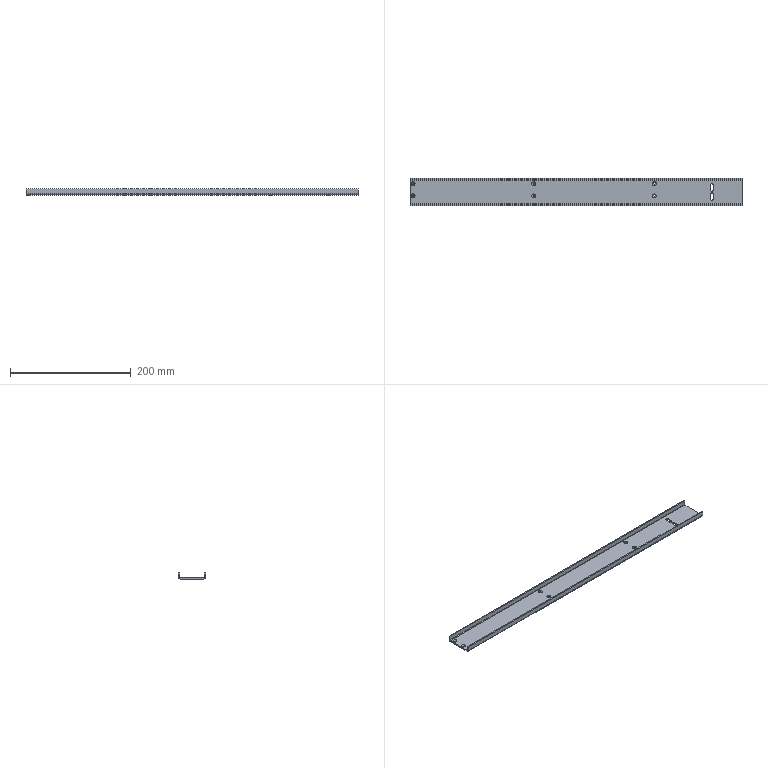Part | SolidWorks | features EdgeFlange 1, FlatPattern 1, HoleWzd 1, ICE 1, SMBaseFlange 1, SheetMetal 1 | 1 solid | 54 faces | box 550 x 45 x 10 mm | volume 65036 mm3 | plane 22 | cylinder 20 | cone 12 | commonest cylinder face diameters 3.4 x12 4.5 x4 1.473 x2 5.473 x2
STEP:
#1=CARTESIAN_POINT('',(-271.7,13.5,-1.6));
#2=VERTEX_POINT('',#1);
#3=CARTESIAN_POINT('',(-268.3,13.5,-1.6));
#4=VERTEX_POINT('',#3);
#5=CARTESIAN_POINT('',(-270.,13.5,-1.6));
#6=DIRECTION('',(0.,0.,1.));
#7=DIRECTION('',(1.,0.,0.));
#8=AXIS2_PLACEMENT_3D('',#5,#6,#7);
#9=CIRCLE('',#8,1.7);
#10=EDGE_CURVE('',#2,#4,#9,.T.);
#11=ORIENTED_EDGE('',*,*,#10,.F.);
#12=CARTESIAN_POINT('',(-273.3,13.5,0.));
#13=VERTEX_POINT('',#12);
#14=CARTESIAN_POINT('',(-273.3,13.5,0.));
#15=DIRECTION('',(-0.7071,0.,0.7071));
#16=VECTOR('',#15,1000.);
#17=LINE('',#14,#16);
#18=EDGE_CURVE('',#2,#13,#17,.T.);
#19=ORIENTED_EDGE('',*,*,#18,.T.);
#20=CARTESIAN_POINT('',(-266.7,13.5,0.));
#21=VERTEX_POINT('',#20);
#22=CARTESIAN_POINT('',(-270.,13.5,0.));
#23=DIRECTION('',(0.,0.,1.));
#24=DIRECTION('',(1.,0.,0.));
#25=AXIS2_PLACEMENT_3D('',#22,#23,#24);
#26=CIRCLE('',#25,3.3);
#27=EDGE_CURVE('',#13,#21,#26,.T.);
#28=ORIENTED_EDGE('',*,*,#27,.T.);
#29=CARTESIAN_POINT('',(-266.7,13.5,0.));
#30=DIRECTION('',(0.7071,0.,0.7071));
#31=VECTOR('',#30,1000.);
#32=LINE('',#29,#31);
#33=EDGE_CURVE('',#4,#21,#32,.T.);
#34=ORIENTED_EDGE('',*,*,#33,.F.);
#35=EDGE_LOOP('',(#11,#19,#28,#34));
#36=FACE_OUTER_BOUND('',#35,.T.);
#37=CARTESIAN_POINT('',(-270.,13.5,0.));
#38=DIRECTION('',(0.,0.,1.));
#39=DIRECTION('',(1.,0.,0.));
#40=AXIS2_PLACEMENT_3D('',#37,#38,#39);
#41=CONICAL_SURFACE('',#40,3.3,0.7854);
#42=ADVANCED_FACE('',(#36),#41,.F.);
#43=CARTESIAN_POINT('',(-271.7,13.5,-2.));
#44=VERTEX_POINT('',#43);
#45=CARTESIAN_POINT('',(-268.3,13.5,-2.));
#46=VERTEX_POINT('',#45);
#47=CARTESIAN_POINT('',(-270.,13.5,-2.));
#48=DIRECTION('',(0.,0.,1.));
#49=DIRECTION('',(1.,0.,0.));
#50=AXIS2_PLACEMENT_3D('',#47,#48,#49);
#51=CIRCLE('',#50,1.7);
#52=EDGE_CURVE('',#44,#46,#51,.T.);
#53=ORIENTED_EDGE('',*,*,#52,.F.);
#54=CARTESIAN_POINT('',(-271.7,13.5,0.));
#55=DIRECTION('',(0.,0.,1.));
#56=VECTOR('',#55,1000.);
#57=LINE('',#54,#56);
#58=EDGE_CURVE('',#44,#2,#57,.T.);
#59=ORIENTED_EDGE('',*,*,#58,.T.);
#60=ORIENTED_EDGE('',*,*,#10,.T.);
#61=CARTESIAN_POINT('',(-268.3,13.5,0.));
#62=DIRECTION('',(0.,0.,1.));
#63=VECTOR('',#62,1000.);
#64=LINE('',#61,#63);
#65=EDGE_CURVE('',#46,#4,#64,.T.);
#66=ORIENTED_EDGE('',*,*,#65,.F.);
#67=EDGE_LOOP('',(#53,#59,#60,#66));
#68=FACE_OUTER_BOUND('',#67,.T.);
#69=CARTESIAN_POINT('',(-270.,13.5,0.));
#70=DIRECTION('',(0.,0.,1.));
#71=DIRECTION('',(1.,0.,0.));
#72=AXIS2_PLACEMENT_3D('',#69,#70,#71);
#73=CYLINDRICAL_SURFACE('',#72,1.7);
#74=ADVANCED_FACE('',(#68),#73,.F.);
#75=CARTESIAN_POINT('',(-271.7,-6.5,-1.6));
#76=VERTEX_POINT('',#75);
#77=CARTESIAN_POINT('',(-268.3,-6.5,-1.6));
#78=VERTEX_POINT('',#77);
#79=CARTESIAN_POINT('',(-270.,-6.5,-1.6));
#80=DIRECTION('',(0.,0.,1.));
#81=DIRECTION('',(1.,0.,0.));
#82=AXIS2_PLACEMENT_3D('',#79,#80,#81);
#83=CIRCLE('',#82,1.7);
#84=EDGE_CURVE('',#76,#78,#83,.T.);
#85=ORIENTED_EDGE('',*,*,#84,.F.);
#86=CARTESIAN_POINT('',(-273.3,-6.5,0.));
#87=VERTEX_POINT('',#86);
#88=CARTESIAN_POINT('',(-273.3,-6.5,0.));
#89=DIRECTION('',(-0.7071,0.,0.7071));
#90=VECTOR('',#89,1000.);
#91=LINE('',#88,#90);
#92=EDGE_CURVE('',#76,#87,#91,.T.);
#93=ORIENTED_EDGE('',*,*,#92,.T.);
#94=CARTESIAN_POINT('',(-266.7,-6.5,0.));
#95=VERTEX_POINT('',#94);
#96=CARTESIAN_POINT('',(-270.,-6.5,0.));
#97=DIRECTION('',(0.,0.,1.));
#98=DIRECTION('',(1.,0.,0.));
#99=AXIS2_PLACEMENT_3D('',#96,#97,#98);
#100=CIRCLE('',#99,3.3);
#101=EDGE_CURVE('',#87,#95,#100,.T.);
#102=ORIENTED_EDGE('',*,*,#101,.T.);
#103=CARTESIAN_POINT('',(-266.7,-6.5,0.));
#104=DIRECTION('',(0.7071,0.,0.7071));
#105=VECTOR('',#104,1000.);
#106=LINE('',#103,#105);
#107=EDGE_CURVE('',#78,#95,#106,.T.);
#108=ORIENTED_EDGE('',*,*,#107,.F.);
#109=EDGE_LOOP('',(#85,#93,#102,#108));
#110=FACE_OUTER_BOUND('',#109,.T.);
#111=CARTESIAN_POINT('',(-270.,-6.5,0.));
#112=DIRECTION('',(0.,0.,1.));
#113=DIRECTION('',(1.,0.,0.));
#114=AXIS2_PLACEMENT_3D('',#111,#112,#113);
#115=CONICAL_SURFACE('',#114,3.3,0.7854);
#116=ADVANCED_FACE('',(#110),#115,.F.);
#117=CARTESIAN_POINT('',(-271.7,-6.5,-2.));
#118=VERTEX_POINT('',#117);
#119=CARTESIAN_POINT('',(-268.3,-6.5,-2.));
#120=VERTEX_POINT('',#119);
#121=CARTESIAN_POINT('',(-270.,-6.5,-2.));
#122=DIRECTION('',(0.,0.,1.));
#123=DIRECTION('',(1.,0.,0.));
#124=AXIS2_PLACEMENT_3D('',#121,#122,#123);
#125=CIRCLE('',#124,1.7);
#126=EDGE_CURVE('',#118,#120,#125,.T.);
#127=ORIENTED_EDGE('',*,*,#126,.F.);
#128=CARTESIAN_POINT('',(-271.7,-6.5,0.));
#129=DIRECTION('',(0.,0.,1.));
#130=VECTOR('',#129,1000.);
#131=LINE('',#128,#130);
#132=EDGE_CURVE('',#118,#76,#131,.T.);
#133=ORIENTED_EDGE('',*,*,#132,.T.);
#134=ORIENTED_EDGE('',*,*,#84,.T.);
#135=CARTESIAN_POINT('',(-268.3,-6.5,0.));
#136=DIRECTION('',(0.,0.,1.));
#137=VECTOR('',#136,1000.);
#138=LINE('',#135,#137);
#139=EDGE_CURVE('',#120,#78,#138,.T.);
#140=ORIENTED_EDGE('',*,*,#139,.F.);
#141=EDGE_LOOP('',(#127,#133,#134,#140));
#142=FACE_OUTER_BOUND('',#141,.T.);
#143=CARTESIAN_POINT('',(-270.,-6.5,0.));
#144=DIRECTION('',(0.,0.,1.));
#145=DIRECTION('',(1.,0.,0.));
#146=AXIS2_PLACEMENT_3D('',#143,#144,#145);
#147=CYLINDRICAL_SURFACE('',#146,1.7);
#148=ADVANCED_FACE('',(#142),#147,.F.);
#149=CARTESIAN_POINT('',(-71.7,-6.5,-1.6));
#150=VERTEX_POINT('',#149);
#151=CARTESIAN_POINT('',(-68.3,-6.5,-1.6));
#152=VERTEX_POINT('',#151);
#153=CARTESIAN_POINT('',(-70.,-6.5,-1.6));
#154=DIRECTION('',(0.,0.,1.));
#155=DIRECTION('',(1.,0.,0.));
#156=AXIS2_PLACEMENT_3D('',#153,#154,#155);
#157=CIRCLE('',#156,1.7);
#158=EDGE_CURVE('',#150,#152,#157,.T.);
#159=ORIENTED_EDGE('',*,*,#158,.F.);
#160=CARTESIAN_POINT('',(-73.3,-6.5,0.));
#161=VERTEX_POINT('',#160);
#162=CARTESIAN_POINT('',(-73.3,-6.5,0.));
#163=DIRECTION('',(-0.7071,0.,0.7071));
#164=VECTOR('',#163,1000.);
#165=LINE('',#162,#164);
#166=EDGE_CURVE('',#150,#161,#165,.T.);
#167=ORIENTED_EDGE('',*,*,#166,.T.);
#168=CARTESIAN_POINT('',(-66.7,-6.5,0.));
#169=VERTEX_POINT('',#168);
#170=CARTESIAN_POINT('',(-70.,-6.5,0.));
#171=DIRECTION('',(0.,0.,1.));
#172=DIRECTION('',(1.,0.,0.));
#173=AXIS2_PLACEMENT_3D('',#170,#171,#172);
#174=CIRCLE('',#173,3.3);
#175=EDGE_CURVE('',#161,#169,#174,.T.);
#176=ORIENTED_EDGE('',*,*,#175,.T.);
#177=CARTESIAN_POINT('',(-66.7,-6.5,0.));
#178=DIRECTION('',(0.7071,0.,0.7071));
#179=VECTOR('',#178,1000.);
#180=LINE('',#177,#179);
#181=EDGE_CURVE('',#152,#169,#180,.T.);
#182=ORIENTED_EDGE('',*,*,#181,.F.);
#183=EDGE_LOOP('',(#159,#167,#176,#182));
#184=FACE_OUTER_BOUND('',#183,.T.);
#185=CARTESIAN_POINT('',(-70.,-6.5,0.));
#186=DIRECTION('',(0.,0.,1.));
#187=DIRECTION('',(1.,0.,0.));
#188=AXIS2_PLACEMENT_3D('',#185,#186,#187);
#189=CONICAL_SURFACE('',#188,3.3,0.7854);
#190=ADVANCED_FACE('',(#184),#189,.F.);
#191=CARTESIAN_POINT('',(-71.7,-6.5,-2.));
#192=VERTEX_POINT('',#191);
#193=CARTESIAN_POINT('',(-68.3,-6.5,-2.));
#194=VERTEX_POINT('',#193);
#195=CARTESIAN_POINT('',(-70.,-6.5,-2.));
#196=DIRECTION('',(0.,0.,1.));
#197=DIRECTION('',(1.,0.,0.));
#198=AXIS2_PLACEMENT_3D('',#195,#196,#197);
#199=CIRCLE('',#198,1.7);
#200=EDGE_CURVE('',#192,#194,#199,.T.);
#201=ORIENTED_EDGE('',*,*,#200,.F.);
#202=CARTESIAN_POINT('',(-71.7,-6.5,0.));
#203=DIRECTION('',(0.,0.,1.));
#204=VECTOR('',#203,1000.);
#205=LINE('',#202,#204);
#206=EDGE_CURVE('',#192,#150,#205,.T.);
#207=ORIENTED_EDGE('',*,*,#206,.T.);
#208=ORIENTED_EDGE('',*,*,#158,.T.);
#209=CARTESIAN_POINT('',(-68.3,-6.5,0.));
#210=DIRECTION('',(0.,0.,1.));
#211=VECTOR('',#210,1000.);
#212=LINE('',#209,#211);
#213=EDGE_CURVE('',#194,#152,#212,.T.);
#214=ORIENTED_EDGE('',*,*,#213,.F.);
#215=EDGE_LOOP('',(#201,#207,#208,#214));
#216=FACE_OUTER_BOUND('',#215,.T.);
#217=CARTESIAN_POINT('',(-70.,-6.5,0.));
#218=DIRECTION('',(0.,0.,1.));
#219=DIRECTION('',(1.,0.,0.));
#220=AXIS2_PLACEMENT_3D('',#217,#218,#219);
#221=CYLINDRICAL_SURFACE('',#220,1.7);
#222=ADVANCED_FACE('',(#216),#221,.F.);
#223=CARTESIAN_POINT('',(-71.7,13.5,-1.6));
#224=VERTEX_POINT('',#223);
#225=CARTESIAN_POINT('',(-68.3,13.5,-1.6));
#226=VERTEX_POINT('',#225);
#227=CARTESIAN_POINT('',(-70.,13.5,-1.6));
#228=DIRECTION('',(0.,0.,1.));
#229=DIRECTION('',(1.,0.,0.));
#230=AXIS2_PLACEMENT_3D('',#227,#228,#229);
#231=CIRCLE('',#230,1.7);
#232=EDGE_CURVE('',#224,#226,#231,.T.);
#233=ORIENTED_EDGE('',*,*,#232,.F.);
#234=CARTESIAN_POINT('',(-73.3,13.5,0.));
#235=VERTEX_POINT('',#234);
#236=CARTESIAN_POINT('',(-73.3,13.5,0.));
#237=DIRECTION('',(-0.7071,0.,0.7071));
#238=VECTOR('',#237,1000.);
#239=LINE('',#236,#238);
#240=EDGE_CURVE('',#224,#235,#239,.T.);
#241=ORIENTED_EDGE('',*,*,#240,.T.);
#242=CARTESIAN_POINT('',(-66.7,13.5,0.));
#243=VERTEX_POINT('',#242);
#244=CARTESIAN_POINT('',(-70.,13.5,0.));
#245=DIRECTION('',(0.,0.,1.));
#246=DIRECTION('',(1.,0.,0.));
#247=AXIS2_PLACEMENT_3D('',#244,#245,#246);
#248=CIRCLE('',#247,3.3);
#249=EDGE_CURVE('',#235,#243,#248,.T.);
#250=ORIENTED_EDGE('',*,*,#249,.T.);
#251=CARTESIAN_POINT('',(-66.7,13.5,0.));
#252=DIRECTION('',(0.7071,0.,0.7071));
#253=VECTOR('',#252,1000.);
#254=LINE('',#251,#253);
#255=EDGE_CURVE('',#226,#243,#254,.T.);
#256=ORIENTED_EDGE('',*,*,#255,.F.);
#257=EDGE_LOOP('',(#233,#241,#250,#256));
#258=FACE_OUTER_BOUND('',#257,.T.);
#259=CARTESIAN_POINT('',(-70.,13.5,0.));
#260=DIRECTION('',(0.,0.,1.));
#261=DIRECTION('',(1.,0.,0.));
#262=AXIS2_PLACEMENT_3D('',#259,#260,#261);
#263=CONICAL_SURFACE('',#262,3.3,0.7854);
#264=ADVANCED_FACE('',(#258),#263,.F.);
#265=CARTESIAN_POINT('',(-71.7,13.5,-2.));
#266=VERTEX_POINT('',#265);
#267=CARTESIAN_POINT('',(-68.3,13.5,-2.));
#268=VERTEX_POINT('',#267);
#269=CARTESIAN_POINT('',(-70.,13.5,-2.));
#270=DIRECTION('',(0.,0.,1.));
#271=DIRECTION('',(1.,0.,0.));
#272=AXIS2_PLACEMENT_3D('',#269,#270,#271);
#273=CIRCLE('',#272,1.7);
#274=EDGE_CURVE('',#266,#268,#273,.T.);
#275=ORIENTED_EDGE('',*,*,#274,.F.);
#276=CARTESIAN_POINT('',(-71.7,13.5,0.));
#277=DIRECTION('',(0.,0.,1.));
#278=VECTOR('',#277,1000.);
#279=LINE('',#276,#278);
#280=EDGE_CURVE('',#266,#224,#279,.T.);
#281=ORIENTED_EDGE('',*,*,#280,.T.);
#282=ORIENTED_EDGE('',*,*,#232,.T.);
#283=CARTESIAN_POINT('',(-68.3,13.5,0.));
#284=DIRECTION('',(0.,0.,1.));
#285=VECTOR('',#284,1000.);
#286=LINE('',#283,#285);
#287=EDGE_CURVE('',#268,#226,#286,.T.);
#288=ORIENTED_EDGE('',*,*,#287,.F.);
#289=EDGE_LOOP('',(#275,#281,#282,#288));
#290=FACE_OUTER_BOUND('',#289,.T.);
#291=CARTESIAN_POINT('',(-70.,13.5,0.));
#292=DIRECTION('',(0.,0.,1.));
#293=DIRECTION('',(1.,0.,0.));
#294=AXIS2_PLACEMENT_3D('',#291,#292,#293);
#295=CYLINDRICAL_SURFACE('',#294,1.7);
#296=ADVANCED_FACE('',(#290),#295,.F.);
#297=CARTESIAN_POINT('',(128.3,13.5,-1.6));
#298=VERTEX_POINT('',#297);
#299=CARTESIAN_POINT('',(131.7,13.5,-1.6));
#300=VERTEX_POINT('',#299);
#301=CARTESIAN_POINT('',(130.,13.5,-1.6));
#302=DIRECTION('',(0.,0.,1.));
#303=DIRECTION('',(1.,0.,0.));
#304=AXIS2_PLACEMENT_3D('',#301,#302,#303);
#305=CIRCLE('',#304,1.7);
#306=EDGE_CURVE('',#298,#300,#305,.T.);
#307=ORIENTED_EDGE('',*,*,#306,.F.);
#308=CARTESIAN_POINT('',(126.7,13.5,0.));
#309=VERTEX_POINT('',#308);
#310=CARTESIAN_POINT('',(126.7,13.5,0.));
#311=DIRECTION('',(-0.7071,0.,0.7071));
#312=VECTOR('',#311,1000.);
#313=LINE('',#310,#312);
#314=EDGE_CURVE('',#298,#309,#313,.T.);
#315=ORIENTED_EDGE('',*,*,#314,.T.);
#316=CARTESIAN_POINT('',(133.3,13.5,0.));
#317=VERTEX_POINT('',#316);
#318=CARTESIAN_POINT('',(130.,13.5,0.));
#319=DIRECTION('',(0.,0.,1.));
#320=DIRECTION('',(1.,0.,0.));
#321=AXIS2_PLACEMENT_3D('',#318,#319,#320);
#322=CIRCLE('',#321,3.3);
#323=EDGE_CURVE('',#309,#317,#322,.T.);
#324=ORIENTED_EDGE('',*,*,#323,.T.);
#325=CARTESIAN_POINT('',(133.3,13.5,0.));
#326=DIRECTION('',(0.7071,0.,0.7071));
#327=VECTOR('',#326,1000.);
#328=LINE('',#325,#327);
#329=EDGE_CURVE('',#300,#317,#328,.T.);
#330=ORIENTED_EDGE('',*,*,#329,.F.);
#331=EDGE_LOOP('',(#307,#315,#324,#330));
#332=FACE_OUTER_BOUND('',#331,.T.);
#333=CARTESIAN_POINT('',(130.,13.5,0.));
#334=DIRECTION('',(0.,0.,1.));
#335=DIRECTION('',(1.,0.,0.));
#336=AXIS2_PLACEMENT_3D('',#333,#334,#335);
#337=CONICAL_SURFACE('',#336,3.3,0.7854);
#338=ADVANCED_FACE('',(#332),#337,.F.);
#339=CARTESIAN_POINT('',(128.3,13.5,-2.));
#340=VERTEX_POINT('',#339);
#341=CARTESIAN_POINT('',(131.7,13.5,-2.));
#342=VERTEX_POINT('',#341);
#343=CARTESIAN_POINT('',(130.,13.5,-2.));
#344=DIRECTION('',(0.,0.,1.));
#345=DIRECTION('',(1.,0.,0.));
#346=AXIS2_PLACEMENT_3D('',#343,#344,#345);
#347=CIRCLE('',#346,1.7);
#348=EDGE_CURVE('',#340,#342,#347,.T.);
#349=ORIENTED_EDGE('',*,*,#348,.F.);
#350=CARTESIAN_POINT('',(128.3,13.5,0.));
#351=DIRECTION('',(0.,0.,1.));
#352=VECTOR('',#351,1000.);
#353=LINE('',#350,#352);
#354=EDGE_CURVE('',#340,#298,#353,.T.);
#355=ORIENTED_EDGE('',*,*,#354,.T.);
#356=ORIENTED_EDGE('',*,*,#306,.T.);
#357=CARTESIAN_POINT('',(131.7,13.5,0.));
#358=DIRECTION('',(0.,0.,1.));
#359=VECTOR('',#358,1000.);
#360=LINE('',#357,#359);
#361=EDGE_CURVE('',#342,#300,#360,.T.);
#362=ORIENTED_EDGE('',*,*,#361,.F.);
#363=EDGE_LOOP('',(#349,#355,#356,#362));
#364=FACE_OUTER_BOUND('',#363,.T.);
#365=CARTESIAN_POINT('',(130.,13.5,0.));
#366=DIRECTION('',(0.,0.,1.));
#367=DIRECTION('',(1.,0.,0.));
#368=AXIS2_PLACEMENT_3D('',#365,#366,#367);
#369=CYLINDRICAL_SURFACE('',#368,1.7);
#370=ADVANCED_FACE('',(#364),#369,.F.);
#371=CARTESIAN_POINT('',(128.3,-6.5,-1.6));
#372=VERTEX_POINT('',#371);
#373=CARTESIAN_POINT('',(131.7,-6.5,-1.6));
#374=VERTEX_POINT('',#373);
#375=CARTESIAN_POINT('',(130.,-6.5,-1.6));
#376=DIRECTION('',(0.,0.,1.));
#377=DIRECTION('',(1.,0.,0.));
#378=AXIS2_PLACEMENT_3D('',#375,#376,#377);
#379=CIRCLE('',#378,1.7);
#380=EDGE_CURVE('',#372,#374,#379,.T.);
#381=ORIENTED_EDGE('',*,*,#380,.F.);
#382=CARTESIAN_POINT('',(126.7,-6.5,0.));
#383=VERTEX_POINT('',#382);
#384=CARTESIAN_POINT('',(126.7,-6.5,0.));
#385=DIRECTION('',(-0.7071,0.,0.7071));
#386=VECTOR('',#385,1000.);
#387=LINE('',#384,#386);
#388=EDGE_CURVE('',#372,#383,#387,.T.);
#389=ORIENTED_EDGE('',*,*,#388,.T.);
#390=CARTESIAN_POINT('',(133.3,-6.5,0.));
#391=VERTEX_POINT('',#390);
#392=CARTESIAN_POINT('',(130.,-6.5,0.));
#393=DIRECTION('',(0.,0.,1.));
#394=DIRECTION('',(1.,0.,0.));
#395=AXIS2_PLACEMENT_3D('',#392,#393,#394);
#396=CIRCLE('',#395,3.3);
#397=EDGE_CURVE('',#383,#391,#396,.T.);
#398=ORIENTED_EDGE('',*,*,#397,.T.);
#399=CARTESIAN_POINT('',(133.3,-6.5,0.));
#400=DIRECTION('',(0.7071,0.,0.7071));
#401=VECTOR('',#400,1000.);
#402=LINE('',#399,#401);
#403=EDGE_CURVE('',#374,#391,#402,.T.);
#404=ORIENTED_EDGE('',*,*,#403,.F.);
#405=EDGE_LOOP('',(#381,#389,#398,#404));
#406=FACE_OUTER_BOUND('',#405,.T.);
#407=CARTESIAN_POINT('',(130.,-6.5,0.));
#408=DIRECTION('',(0.,0.,1.));
#409=DIRECTION('',(1.,0.,0.));
#410=AXIS2_PLACEMENT_3D('',#407,#408,#409);
#411=CONICAL_SURFACE('',#410,3.3,0.7854);
#412=ADVANCED_FACE('',(#406),#411,.F.);
#413=CARTESIAN_POINT('',(128.3,-6.5,-2.));
#414=VERTEX_POINT('',#413);
#415=CARTESIAN_POINT('',(131.7,-6.5,-2.));
#416=VERTEX_POINT('',#415);
#417=CARTESIAN_POINT('',(130.,-6.5,-2.));
#418=DIRECTION('',(0.,0.,1.));
#419=DIRECTION('',(1.,0.,0.));
#420=AXIS2_PLACEMENT_3D('',#417,#418,#419);
#421=CIRCLE('',#420,1.7);
#422=EDGE_CURVE('',#414,#416,#421,.T.);
#423=ORIENTED_EDGE('',*,*,#422,.F.);
#424=CARTESIAN_POINT('',(128.3,-6.5,0.));
#425=DIRECTION('',(0.,0.,1.));
#426=VECTOR('',#425,1000.);
#427=LINE('',#424,#426);
#428=EDGE_CURVE('',#414,#372,#427,.T.);
#429=ORIENTED_EDGE('',*,*,#428,.T.);
#430=ORIENTED_EDGE('',*,*,#380,.T.);
#431=CARTESIAN_POINT('',(131.7,-6.5,0.));
#432=DIRECTION('',(0.,0.,1.));
#433=VECTOR('',#432,1000.);
#434=LINE('',#431,#433);
#435=EDGE_CURVE('',#416,#374,#434,.T.);
#436=ORIENTED_EDGE('',*,*,#435,.F.);
#437=EDGE_LOOP('',(#423,#429,#430,#436));
#438=FACE_OUTER_BOUND('',#437,.T.);
#439=CARTESIAN_POINT('',(130.,-6.5,0.));
#440=DIRECTION('',(0.,0.,1.));
#441=DIRECTION('',(1.,0.,0.));
#442=AXIS2_PLACEMENT_3D('',#439,#440,#441);
#443=CYLINDRICAL_SURFACE('',#442,1.7);
#444=ADVANCED_FACE('',(#438),#443,.F.);
#445=CARTESIAN_POINT('',(-270.,13.5,-2.));
#446=DIRECTION('',(0.,0.,1.));
#447=DIRECTION('',(1.,0.,0.));
#448=AXIS2_PLACEMENT_3D('',#445,#446,#447);
#449=CIRCLE('',#448,1.7);
#450=EDGE_CURVE('',#46,#44,#449,.T.);
#451=ORIENTED_EDGE('',*,*,#450,.T.);
#452=ORIENTED_EDGE('',*,*,#52,.T.);
#453=EDGE_LOOP('',(#451,#452));
#454=FACE_BOUND('',#453,.T.);
#455=CARTESIAN_POINT('',(-270.,-6.5,-2.));
#456=DIRECTION('',(0.,0.,1.));
#457=DIRECTION('',(1.,0.,0.));
#458=AXIS2_PLACEMENT_3D('',#455,#456,#457);
#459=CIRCLE('',#458,1.7);
#460=EDGE_CURVE('',#120,#118,#459,.T.);
#461=ORIENTED_EDGE('',*,*,#460,.T.);
#462=ORIENTED_EDGE('',*,*,#126,.T.);
#463=EDGE_LOOP('',(#461,#462));
#464=FACE_BOUND('',#463,.T.);
#465=CARTESIAN_POINT('',(-70.,-6.5,-2.));
#466=DIRECTION('',(0.,0.,1.));
#467=DIRECTION('',(1.,0.,0.));
#468=AXIS2_PLACEMENT_3D('',#465,#466,#467);
#469=CIRCLE('',#468,1.7);
#470=EDGE_CURVE('',#194,#192,#469,.T.);
#471=ORIENTED_EDGE('',*,*,#470,.T.);
#472=ORIENTED_EDGE('',*,*,#200,.T.);
#473=EDGE_LOOP('',(#471,#472));
#474=FACE_BOUND('',#473,.T.);
#475=CARTESIAN_POINT('',(-70.,13.5,-2.));
#476=DIRECTION('',(0.,0.,1.));
#477=DIRECTION('',(1.,0.,0.));
#478=AXIS2_PLACEMENT_3D('',#475,#476,#477);
#479=CIRCLE('',#478,1.7);
#480=EDGE_CURVE('',#268,#266,#479,.T.);
#481=ORIENTED_EDGE('',*,*,#480,.T.);
#482=ORIENTED_EDGE('',*,*,#274,.T.);
#483=EDGE_LOOP('',(#481,#482));
#484=FACE_BOUND('',#483,.T.);
#485=CARTESIAN_POINT('',(130.,13.5,-2.));
#486=DIRECTION('',(0.,0.,1.));
#487=DIRECTION('',(1.,0.,0.));
#488=AXIS2_PLACEMENT_3D('',#485,#486,#487);
#489=CIRCLE('',#488,1.7);
#490=EDGE_CURVE('',#342,#340,#489,.T.);
#491=ORIENTED_EDGE('',*,*,#490,.T.);
#492=ORIENTED_EDGE('',*,*,#348,.T.);
#493=EDGE_LOOP('',(#491,#492));
#494=FACE_BOUND('',#493,.T.);
#495=CARTESIAN_POINT('',(130.,-6.5,-2.));
#496=DIRECTION('',(0.,0.,1.));
#497=DIRECTION('',(1.,0.,0.));
#498=AXIS2_PLACEMENT_3D('',#495,#496,#497);
#499=CIRCLE('',#498,1.7);
#500=EDGE_CURVE('',#416,#414,#499,.T.);
#501=ORIENTED_EDGE('',*,*,#500,.T.);
#502=ORIENTED_EDGE('',*,*,#422,.T.);
#503=EDGE_LOOP('',(#501,#502));
#504=FACE_BOUND('',#503,.T.);
#505=CARTESIAN_POINT('',(227.25,-11.5,-2.));
#506=VERTEX_POINT('',#505);
#507=CARTESIAN_POINT('',(227.25,-3.5,-2.));
#508=VERTEX_POINT('',#507);
#509=CARTESIAN_POINT('',(227.25,0.,-2.));
#510=DIRECTION('',(0.,1.,0.));
#511=VECTOR('',#510,1000.);
#512=LINE('',#509,#511);
#513=EDGE_CURVE('',#506,#508,#512,.T.);
#514=ORIENTED_EDGE('',*,*,#513,.T.);
#515=CARTESIAN_POINT('',(222.75,-3.5,-2.));
#516=VERTEX_POINT('',#515);
#517=CARTESIAN_POINT('',(225.,-3.5,-2.));
#518=DIRECTION('',(0.,0.,1.));
#519=DIRECTION('',(1.,0.,0.));
#520=AXIS2_PLACEMENT_3D('',#517,#518,#519);
#521=CIRCLE('',#520,2.25);
#522=EDGE_CURVE('',#508,#516,#521,.T.);
#523=ORIENTED_EDGE('',*,*,#522,.T.);
#524=CARTESIAN_POINT('',(222.75,-11.5,-2.));
#525=VERTEX_POINT('',#524);
#526=CARTESIAN_POINT('',(222.75,0.,-2.));
#527=DIRECTION('',(0.,-1.,0.));
#528=VECTOR('',#527,1000.);
#529=LINE('',#526,#528);
#530=EDGE_CURVE('',#516,#525,#529,.T.);
#531=ORIENTED_EDGE('',*,*,#530,.T.);
#532=CARTESIAN_POINT('',(225.,-11.5,-2.));
#533=DIRECTION('',(0.,0.,1.));
#534=DIRECTION('',(1.,0.,0.));
#535=AXIS2_PLACEMENT_3D('',#532,#533,#534);
#536=CIRCLE('',#535,2.25);
#537=EDGE_CURVE('',#525,#506,#536,.T.);
#538=ORIENTED_EDGE('',*,*,#537,.T.);
#539=EDGE_LOOP('',(#514,#523,#531,#538));
#540=FACE_BOUND('',#539,.T.);
#541=CARTESIAN_POINT('',(227.25,3.5,-2.));
#542=VERTEX_POINT('',#541);
#543=CARTESIAN_POINT('',(227.25,11.5,-2.));
#544=VERTEX_POINT('',#543);
#545=CARTESIAN_POINT('',(227.25,0.,-2.));
#546=DIRECTION('',(0.,1.,0.));
#547=VECTOR('',#546,1000.);
#548=LINE('',#545,#547);
#549=EDGE_CURVE('',#542,#544,#548,.T.);
#550=ORIENTED_EDGE('',*,*,#549,.T.);
#551=CARTESIAN_POINT('',(222.75,11.5,-2.));
#552=VERTEX_POINT('',#551);
#553=CARTESIAN_POINT('',(225.,11.5,-2.));
#554=DIRECTION('',(0.,0.,1.));
#555=DIRECTION('',(1.,0.,0.));
#556=AXIS2_PLACEMENT_3D('',#553,#554,#555);
#557=CIRCLE('',#556,2.25);
#558=EDGE_CURVE('',#544,#552,#557,.T.);
#559=ORIENTED_EDGE('',*,*,#558,.T.);
#560=CARTESIAN_POINT('',(222.75,3.5,-2.));
#561=VERTEX_POINT('',#560);
#562=CARTESIAN_POINT('',(222.75,0.,-2.));
#563=DIRECTION('',(0.,-1.,0.));
#564=VECTOR('',#563,1000.);
#565=LINE('',#562,#564);
#566=EDGE_CURVE('',#552,#561,#565,.T.);
#567=ORIENTED_EDGE('',*,*,#566,.T.);
#568=CARTESIAN_POINT('',(225.,3.5,-2.));
#569=DIRECTION('',(0.,0.,1.));
#570=DIRECTION('',(1.,0.,0.));
#571=AXIS2_PLACEMENT_3D('',#568,#569,#570);
#572=CIRCLE('',#571,2.25);
#573=EDGE_CURVE('',#561,#542,#572,.T.);
#574=ORIENTED_EDGE('',*,*,#573,.T.);
#575=EDGE_LOOP('',(#550,#559,#567,#574));
#576=FACE_BOUND('',#575,.T.);
#577=CARTESIAN_POINT('',(-275.,19.763,-2.));
#578=VERTEX_POINT('',#577);
#579=CARTESIAN_POINT('',(275.,19.763,-2.));
#580=VERTEX_POINT('',#579);
#581=CARTESIAN_POINT('',(-275.,19.763,-2.));
#582=DIRECTION('',(1.,0.,0.));
#583=VECTOR('',#582,1000.);
#584=LINE('',#581,#583);
#585=EDGE_CURVE('',#578,#580,#584,.T.);
#586=ORIENTED_EDGE('',*,*,#585,.T.);
#587=CARTESIAN_POINT('',(275.,-19.763,-2.));
#588=VERTEX_POINT('',#587);
#589=CARTESIAN_POINT('',(275.,22.5,-2.));
#590=DIRECTION('',(0.,1.,0.));
#591=VECTOR('',#590,1000.);
#592=LINE('',#589,#591);
#593=EDGE_CURVE('',#588,#580,#592,.T.);
#594=ORIENTED_EDGE('',*,*,#593,.F.);
#595=CARTESIAN_POINT('',(-275.,-19.763,-2.));
#596=VERTEX_POINT('',#595);
#597=CARTESIAN_POINT('',(275.,-19.763,-2.));
#598=DIRECTION('',(-1.,0.,0.));
#599=VECTOR('',#598,1000.);
#600=LINE('',#597,#599);
#601=EDGE_CURVE('',#588,#596,#600,.T.);
#602=ORIENTED_EDGE('',*,*,#601,.T.);
#603=CARTESIAN_POINT('',(-275.,22.5,-2.));
#604=DIRECTION('',(0.,-1.,0.));
#605=VECTOR('',#604,1000.);
#606=LINE('',#603,#605);
#607=EDGE_CURVE('',#578,#596,#606,.T.);
#608=ORIENTED_EDGE('',*,*,#607,.F.);
#609=EDGE_LOOP('',(#586,#594,#602,#608));
#610=FACE_OUTER_BOUND('',#609,.T.);
#611=CARTESIAN_POINT('',(0.,0.,-2.));
#612=DIRECTION('',(0.,0.,1.));
#613=DIRECTION('',(1.,0.,0.));
#614=AXIS2_PLACEMENT_3D('',#611,#612,#613);
#615=PLANE('',#614);
#616=ADVANCED_FACE('',(#454,#464,#474,#484,#494,#504,#540,#576,#610),#615,.F.);
#617=CARTESIAN_POINT('',(-270.,13.5,0.));
#618=DIRECTION('',(0.,0.,1.));
#619=DIRECTION('',(1.,0.,0.));
#620=AXIS2_PLACEMENT_3D('',#617,#618,#619);
#621=CIRCLE('',#620,3.3);
#622=EDGE_CURVE('',#21,#13,#621,.T.);
#623=ORIENTED_EDGE('',*,*,#622,.F.);
#624=ORIENTED_EDGE('',*,*,#27,.F.);
#625=EDGE_LOOP('',(#623,#624));
#626=FACE_BOUND('',#625,.T.);
#627=CARTESIAN_POINT('',(-270.,-6.5,0.));
#628=DIRECTION('',(0.,0.,1.));
#629=DIRECTION('',(1.,0.,0.));
#630=AXIS2_PLACEMENT_3D('',#627,#628,#629);
#631=CIRCLE('',#630,3.3);
#632=EDGE_CURVE('',#95,#87,#631,.T.);
#633=ORIENTED_EDGE('',*,*,#632,.F.);
#634=ORIENTED_EDGE('',*,*,#101,.F.);
#635=EDGE_LOOP('',(#633,#634));
#636=FACE_BOUND('',#635,.T.);
#637=CARTESIAN_POINT('',(-70.,-6.5,0.));
#638=DIRECTION('',(0.,0.,1.));
#639=DIRECTION('',(1.,0.,0.));
#640=AXIS2_PLACEMENT_3D('',#637,#638,#639);
#641=CIRCLE('',#640,3.3);
#642=EDGE_CURVE('',#169,#161,#641,.T.);
#643=ORIENTED_EDGE('',*,*,#642,.F.);
#644=ORIENTED_EDGE('',*,*,#175,.F.);
#645=EDGE_LOOP('',(#643,#644));
#646=FACE_BOUND('',#645,.T.);
#647=CARTESIAN_POINT('',(-70.,13.5,0.));
#648=DIRECTION('',(0.,0.,1.));
#649=DIRECTION('',(1.,0.,0.));
#650=AXIS2_PLACEMENT_3D('',#647,#648,#649);
#651=CIRCLE('',#650,3.3);
#652=EDGE_CURVE('',#243,#235,#651,.T.);
#653=ORIENTED_EDGE('',*,*,#652,.F.);
#654=ORIENTED_EDGE('',*,*,#249,.F.);
#655=EDGE_LOOP('',(#653,#654));
#656=FACE_BOUND('',#655,.T.);
#657=CARTESIAN_POINT('',(130.,13.5,0.));
#658=DIRECTION('',(0.,0.,1.));
#659=DIRECTION('',(1.,0.,0.));
#660=AXIS2_PLACEMENT_3D('',#657,#658,#659);
#661=CIRCLE('',#660,3.3);
#662=EDGE_CURVE('',#317,#309,#661,.T.);
#663=ORIENTED_EDGE('',*,*,#662,.F.);
#664=ORIENTED_EDGE('',*,*,#323,.F.);
#665=EDGE_LOOP('',(#663,#664));
#666=FACE_BOUND('',#665,.T.);
#667=CARTESIAN_POINT('',(130.,-6.5,0.));
#668=DIRECTION('',(0.,0.,1.));
#669=DIRECTION('',(1.,0.,0.));
#670=AXIS2_PLACEMENT_3D('',#667,#668,#669);
#671=CIRCLE('',#670,3.3);
#672=EDGE_CURVE('',#391,#383,#671,.T.);
#673=ORIENTED_EDGE('',*,*,#672,.F.);
#674=ORIENTED_EDGE('',*,*,#397,.F.);
#675=EDGE_LOOP('',(#673,#674));
#676=FACE_BOUND('',#675,.T.);
#677=CARTESIAN_POINT('',(227.25,-3.5,0.));
#678=VERTEX_POINT('',#677);
#679=CARTESIAN_POINT('',(222.75,-3.5,0.));
#680=VERTEX_POINT('',#679);
#681=CARTESIAN_POINT('',(225.,-3.5,0.));
#682=DIRECTION('',(0.,0.,1.));
#683=DIRECTION('',(1.,0.,0.));
#684=AXIS2_PLACEMENT_3D('',#681,#682,#683);
#685=CIRCLE('',#684,2.25);
#686=EDGE_CURVE('',#678,#680,#685,.T.);
#687=ORIENTED_EDGE('',*,*,#686,.F.);
#688=CARTESIAN_POINT('',(227.25,-11.5,0.));
#689=VERTEX_POINT('',#688);
#690=CARTESIAN_POINT('',(227.25,-3.5,0.));
#691=DIRECTION('',(0.,1.,0.));
#692=VECTOR('',#691,1000.);
#693=LINE('',#690,#692);
#694=EDGE_CURVE('',#689,#678,#693,.T.);
#695=ORIENTED_EDGE('',*,*,#694,.F.);
#696=CARTESIAN_POINT('',(222.75,-11.5,0.));
#697=VERTEX_POINT('',#696);
#698=CARTESIAN_POINT('',(225.,-11.5,0.));
#699=DIRECTION('',(0.,0.,1.));
#700=DIRECTION('',(1.,0.,0.));
#701=AXIS2_PLACEMENT_3D('',#698,#699,#700);
#702=CIRCLE('',#701,2.25);
#703=EDGE_CURVE('',#697,#689,#702,.T.);
#704=ORIENTED_EDGE('',*,*,#703,.F.);
#705=CARTESIAN_POINT('',(222.75,-3.5,0.));
#706=DIRECTION('',(0.,-1.,0.));
#707=VECTOR('',#706,1000.);
#708=LINE('',#705,#707);
#709=EDGE_CURVE('',#680,#697,#708,.T.);
#710=ORIENTED_EDGE('',*,*,#709,.F.);
#711=EDGE_LOOP('',(#687,#695,#704,#710));
#712=FACE_BOUND('',#711,.T.);
#713=CARTESIAN_POINT('',(227.25,11.5,0.));
#714=VERTEX_POINT('',#713);
#715=CARTESIAN_POINT('',(222.75,11.5,0.));
#716=VERTEX_POINT('',#715);
#717=CARTESIAN_POINT('',(225.,11.5,0.));
#718=DIRECTION('',(0.,0.,1.));
#719=DIRECTION('',(1.,0.,0.));
#720=AXIS2_PLACEMENT_3D('',#717,#718,#719);
#721=CIRCLE('',#720,2.25);
#722=EDGE_CURVE('',#714,#716,#721,.T.);
#723=ORIENTED_EDGE('',*,*,#722,.F.);
#724=CARTESIAN_POINT('',(227.25,3.5,0.));
#725=VERTEX_POINT('',#724);
#726=CARTESIAN_POINT('',(227.25,11.5,0.));
#727=DIRECTION('',(0.,1.,0.));
#728=VECTOR('',#727,1000.);
#729=LINE('',#726,#728);
#730=EDGE_CURVE('',#725,#714,#729,.T.);
#731=ORIENTED_EDGE('',*,*,#730,.F.);
#732=CARTESIAN_POINT('',(222.75,3.5,0.));
#733=VERTEX_POINT('',#732);
#734=CARTESIAN_POINT('',(225.,3.5,0.));
#735=DIRECTION('',(0.,0.,1.));
#736=DIRECTION('',(1.,0.,0.));
#737=AXIS2_PLACEMENT_3D('',#734,#735,#736);
#738=CIRCLE('',#737,2.25);
#739=EDGE_CURVE('',#733,#725,#738,.T.);
#740=ORIENTED_EDGE('',*,*,#739,.F.);
#741=CARTESIAN_POINT('',(222.75,11.5,0.));
#742=DIRECTION('',(0.,-1.,0.));
#743=VECTOR('',#742,1000.);
#744=LINE('',#741,#743);
#745=EDGE_CURVE('',#716,#733,#744,.T.);
#746=ORIENTED_EDGE('',*,*,#745,.F.);
#747=EDGE_LOOP('',(#723,#731,#740,#746));
#748=FACE_BOUND('',#747,.T.);
#749=CARTESIAN_POINT('',(275.,-19.763,0.));
#750=VERTEX_POINT('',#749);
#751=CARTESIAN_POINT('',(275.,19.763,0.));
#752=VERTEX_POINT('',#751);
#753=CARTESIAN_POINT('',(275.,22.5,0.));
#754=DIRECTION('',(0.,1.,0.));
#755=VECTOR('',#754,1000.);
#756=LINE('',#753,#755);
#757=EDGE_CURVE('',#750,#752,#756,.T.);
#758=ORIENTED_EDGE('',*,*,#757,.T.);
#759=CARTESIAN_POINT('',(-275.,19.763,0.));
#760=VERTEX_POINT('',#759);
#761=CARTESIAN_POINT('',(-275.,19.763,0.));
#762=DIRECTION('',(1.,0.,0.));
#763=VECTOR('',#762,1000.);
#764=LINE('',#761,#763);
#765=EDGE_CURVE('',#760,#752,#764,.T.);
#766=ORIENTED_EDGE('',*,*,#765,.F.);
#767=CARTESIAN_POINT('',(-275.,-19.763,0.));
#768=VERTEX_POINT('',#767);
#769=CARTESIAN_POINT('',(-275.,22.5,0.));
#770=DIRECTION('',(0.,-1.,0.));
#771=VECTOR('',#770,1000.);
#772=LINE('',#769,#771);
#773=EDGE_CURVE('',#760,#768,#772,.T.);
#774=ORIENTED_EDGE('',*,*,#773,.T.);
#775=CARTESIAN_POINT('',(275.,-19.763,0.));
#776=DIRECTION('',(-1.,0.,0.));
#777=VECTOR('',#776,1000.);
#778=LINE('',#775,#777);
#779=EDGE_CURVE('',#750,#768,#778,.T.);
#780=ORIENTED_EDGE('',*,*,#779,.F.);
#781=EDGE_LOOP('',(#758,#766,#774,#780));
#782=FACE_OUTER_BOUND('',#781,.T.);
#783=CARTESIAN_POINT('',(0.,0.,0.));
#784=DIRECTION('',(0.,0.,1.));
#785=DIRECTION('',(1.,0.,0.));
#786=AXIS2_PLACEMENT_3D('',#783,#784,#785);
#787=PLANE('',#786);
#788=ADVANCED_FACE('',(#626,#636,#646,#656,#666,#676,#712,#748,#782),#787,.T.);
#789=ORIENTED_EDGE('',*,*,#773,.F.);
#790=CARTESIAN_POINT('',(-275.,19.763,0.));
#791=DIRECTION('',(0.,0.,-1.));
#792=VECTOR('',#791,1000.);
#793=LINE('',#790,#792);
#794=EDGE_CURVE('',#760,#578,#793,.T.);
#795=ORIENTED_EDGE('',*,*,#794,.T.);
#796=ORIENTED_EDGE('',*,*,#607,.T.);
#797=CARTESIAN_POINT('',(-275.,-19.763,0.));
#798=DIRECTION('',(0.,0.,-1.));
#799=VECTOR('',#798,1000.);
#800=LINE('',#797,#799);
#801=EDGE_CURVE('',#768,#596,#800,.T.);
#802=ORIENTED_EDGE('',*,*,#801,.F.);
#803=EDGE_LOOP('',(#789,#795,#796,#802));
#804=FACE_OUTER_BOUND('',#803,.T.);
#805=CARTESIAN_POINT('',(-275.,22.5,-2.));
#806=DIRECTION('',(-1.,0.,0.));
#807=DIRECTION('',(0.,0.,1.));
#808=AXIS2_PLACEMENT_3D('',#805,#806,#807);
#809=PLANE('',#808);
#810=ADVANCED_FACE('',(#804),#809,.T.);
#811=CARTESIAN_POINT('',(275.,19.763,0.));
#812=DIRECTION('',(0.,0.,-1.));
#813=VECTOR('',#812,1000.);
#814=LINE('',#811,#813);
#815=EDGE_CURVE('',#752,#580,#814,.T.);
#816=ORIENTED_EDGE('',*,*,#815,.F.);
#817=ORIENTED_EDGE('',*,*,#757,.F.);
#818=CARTESIAN_POINT('',(275.,-19.763,0.));
#819=DIRECTION('',(0.,0.,-1.));
#820=VECTOR('',#819,1000.);
#821=LINE('',#818,#820);
#822=EDGE_CURVE('',#750,#588,#821,.T.);
#823=ORIENTED_EDGE('',*,*,#822,.T.);
#824=ORIENTED_EDGE('',*,*,#593,.T.);
#825=EDGE_LOOP('',(#816,#817,#823,#824));
#826=FACE_OUTER_BOUND('',#825,.T.);
#827=CARTESIAN_POINT('',(275.,22.5,-2.));
#828=DIRECTION('',(1.,0.,0.));
#829=DIRECTION('',(0.,0.,-1.));
#830=AXIS2_PLACEMENT_3D('',#827,#828,#829);
#831=PLANE('',#830);
#832=ADVANCED_FACE('',(#826),#831,.T.);
#833=CARTESIAN_POINT('',(-275.,-20.5,0.7366));
#834=VERTEX_POINT('',#833);
#835=CARTESIAN_POINT('',(-275.,-22.5,0.7366));
#836=VERTEX_POINT('',#835);
#837=CARTESIAN_POINT('',(-275.,-22.5,0.7366));
#838=DIRECTION('',(0.,-1.,0.));
#839=VECTOR('',#838,1000.);
#840=LINE('',#837,#839);
#841=EDGE_CURVE('',#834,#836,#840,.T.);
#842=ORIENTED_EDGE('',*,*,#841,.F.);
#843=CARTESIAN_POINT('',(-275.,-19.763,0.7366));
#844=DIRECTION('',(-1.,0.,0.));
#845=DIRECTION('',(0.,0.,-1.));
#846=AXIS2_PLACEMENT_3D('',#843,#844,#845);
#847=CIRCLE('',#846,0.7366);
#848=EDGE_CURVE('',#768,#834,#847,.T.);
#849=ORIENTED_EDGE('',*,*,#848,.F.);
#850=ORIENTED_EDGE('',*,*,#801,.T.);
#851=CARTESIAN_POINT('',(-275.,-19.763,0.7366));
#852=DIRECTION('',(-1.,0.,0.));
#853=DIRECTION('',(0.,0.,-1.));
#854=AXIS2_PLACEMENT_3D('',#851,#852,#853);
#855=CIRCLE('',#854,2.737);
#856=EDGE_CURVE('',#596,#836,#855,.T.);
#857=ORIENTED_EDGE('',*,*,#856,.T.);
#858=EDGE_LOOP('',(#842,#849,#850,#857));
#859=FACE_OUTER_BOUND('',#858,.T.);
#860=CARTESIAN_POINT('',(-275.,-19.763,0.7366));
#861=DIRECTION('',(-1.,0.,0.));
#862=DIRECTION('',(0.,0.,1.));
#863=AXIS2_PLACEMENT_3D('',#860,#861,#862);
#864=PLANE('',#863);
#865=ADVANCED_FACE('',(#859),#864,.T.);
#866=CARTESIAN_POINT('',(275.,-20.5,0.7366));
#867=VERTEX_POINT('',#866);
#868=CARTESIAN_POINT('',(275.,-19.763,0.7366));
#869=DIRECTION('',(1.,0.,0.));
#870=DIRECTION('',(0.,0.,-1.));
#871=AXIS2_PLACEMENT_3D('',#868,#869,#870);
#872=CIRCLE('',#871,0.7366);
#873=EDGE_CURVE('',#867,#750,#872,.T.);
#874=ORIENTED_EDGE('',*,*,#873,.F.);
#875=CARTESIAN_POINT('',(275.,-22.5,0.7366));
#876=VERTEX_POINT('',#875);
#877=CARTESIAN_POINT('',(275.,-20.5,0.7366));
#878=DIRECTION('',(0.,-1.,0.));
#879=VECTOR('',#878,1000.);
#880=LINE('',#877,#879);
#881=EDGE_CURVE('',#867,#876,#880,.T.);
#882=ORIENTED_EDGE('',*,*,#881,.T.);
#883=CARTESIAN_POINT('',(275.,-19.763,0.7366));
#884=DIRECTION('',(1.,0.,0.));
#885=DIRECTION('',(0.,0.,-1.));
#886=AXIS2_PLACEMENT_3D('',#883,#884,#885);
#887=CIRCLE('',#886,2.737);
#888=EDGE_CURVE('',#876,#588,#887,.T.);
#889=ORIENTED_EDGE('',*,*,#888,.T.);
#890=ORIENTED_EDGE('',*,*,#822,.F.);
#891=EDGE_LOOP('',(#874,#882,#889,#890));
#892=FACE_OUTER_BOUND('',#891,.T.);
#893=CARTESIAN_POINT('',(275.,-19.763,0.7366));
#894=DIRECTION('',(-1.,0.,0.));
#895=DIRECTION('',(0.,0.,1.));
#896=AXIS2_PLACEMENT_3D('',#893,#894,#895);
#897=PLANE('',#896);
#898=ADVANCED_FACE('',(#892),#897,.F.);
#899=ORIENTED_EDGE('',*,*,#601,.F.);
#900=ORIENTED_EDGE('',*,*,#888,.F.);
#901=CARTESIAN_POINT('',(-275.,-22.5,0.7366));
#902=DIRECTION('',(-1.,0.,0.));
#903=VECTOR('',#902,1000.);
#904=LINE('',#901,#903);
#905=EDGE_CURVE('',#876,#836,#904,.T.);
#906=ORIENTED_EDGE('',*,*,#905,.T.);
#907=ORIENTED_EDGE('',*,*,#856,.F.);
#908=EDGE_LOOP('',(#899,#900,#906,#907));
#909=FACE_OUTER_BOUND('',#908,.T.);
#910=CARTESIAN_POINT('',(275.,-19.763,0.7366));
#911=DIRECTION('',(1.,0.,0.));
#912=DIRECTION('',(0.,-1.,0.));
#913=AXIS2_PLACEMENT_3D('',#910,#911,#912);
#914=CYLINDRICAL_SURFACE('',#913,2.737);
#915=ADVANCED_FACE('',(#909),#914,.T.);
#916=ORIENTED_EDGE('',*,*,#779,.T.);
#917=ORIENTED_EDGE('',*,*,#848,.T.);
#918=CARTESIAN_POINT('',(-275.,-20.5,0.7366));
#919=DIRECTION('',(1.,0.,0.));
#920=VECTOR('',#919,1000.);
#921=LINE('',#918,#920);
#922=EDGE_CURVE('',#834,#867,#921,.T.);
#923=ORIENTED_EDGE('',*,*,#922,.T.);
#924=ORIENTED_EDGE('',*,*,#873,.T.);
#925=EDGE_LOOP('',(#916,#917,#923,#924));
#926=FACE_OUTER_BOUND('',#925,.T.);
#927=CARTESIAN_POINT('',(275.,-19.763,0.7366));
#928=DIRECTION('',(1.,0.,0.));
#929=DIRECTION('',(0.,-1.,0.));
#930=AXIS2_PLACEMENT_3D('',#927,#928,#929);
#931=CYLINDRICAL_SURFACE('',#930,0.7366);
#932=ADVANCED_FACE('',(#926),#931,.F.);
#933=ORIENTED_EDGE('',*,*,#841,.T.);
#934=CARTESIAN_POINT('',(-275.,-22.5,8.));
#935=VERTEX_POINT('',#934);
#936=CARTESIAN_POINT('',(-275.,-22.5,0.));
#937=DIRECTION('',(0.,0.,-1.));
#938=VECTOR('',#937,1000.);
#939=LINE('',#936,#938);
#940=EDGE_CURVE('',#935,#836,#939,.T.);
#941=ORIENTED_EDGE('',*,*,#940,.F.);
#942=CARTESIAN_POINT('',(-275.,-20.5,8.));
#943=VERTEX_POINT('',#942);
#944=CARTESIAN_POINT('',(-275.,-22.5,8.));
#945=DIRECTION('',(0.,1.,0.));
#946=VECTOR('',#945,1000.);
#947=LINE('',#944,#946);
#948=EDGE_CURVE('',#935,#943,#947,.T.);
#949=ORIENTED_EDGE('',*,*,#948,.T.);
#950=CARTESIAN_POINT('',(-275.,-20.5,0.));
#951=DIRECTION('',(0.,0.,-1.));
#952=VECTOR('',#951,1000.);
#953=LINE('',#950,#952);
#954=EDGE_CURVE('',#943,#834,#953,.T.);
#955=ORIENTED_EDGE('',*,*,#954,.T.);
#956=EDGE_LOOP('',(#933,#941,#949,#955));
#957=FACE_OUTER_BOUND('',#956,.T.);
#958=CARTESIAN_POINT('',(-275.,-22.5,0.));
#959=DIRECTION('',(1.,0.,0.));
#960=DIRECTION('',(0.,0.,-1.));
#961=AXIS2_PLACEMENT_3D('',#958,#959,#960);
#962=PLANE('',#961);
#963=ADVANCED_FACE('',(#957),#962,.F.);
#964=ORIENTED_EDGE('',*,*,#881,.F.);
#965=CARTESIAN_POINT('',(275.,-20.5,8.));
#966=VERTEX_POINT('',#965);
#967=CARTESIAN_POINT('',(275.,-20.5,8.));
#968=DIRECTION('',(0.,0.,1.));
#969=VECTOR('',#968,1000.);
#970=LINE('',#967,#969);
#971=EDGE_CURVE('',#867,#966,#970,.T.);
#972=ORIENTED_EDGE('',*,*,#971,.T.);
#973=CARTESIAN_POINT('',(275.,-22.5,8.));
#974=VERTEX_POINT('',#973);
#975=CARTESIAN_POINT('',(275.,-22.5,8.));
#976=DIRECTION('',(0.,1.,0.));
#977=VECTOR('',#976,1000.);
#978=LINE('',#975,#977);
#979=EDGE_CURVE('',#974,#966,#978,.T.);
#980=ORIENTED_EDGE('',*,*,#979,.F.);
#981=CARTESIAN_POINT('',(275.,-22.5,0.));
#982=DIRECTION('',(0.,0.,1.));
#983=VECTOR('',#982,1000.);
#984=LINE('',#981,#983);
#985=EDGE_CURVE('',#876,#974,#984,.T.);
#986=ORIENTED_EDGE('',*,*,#985,.F.);
#987=EDGE_LOOP('',(#964,#972,#980,#986));
#988=FACE_OUTER_BOUND('',#987,.T.);
#989=CARTESIAN_POINT('',(275.,-22.5,8.));
#990=DIRECTION('',(-1.,0.,0.));
#991=DIRECTION('',(0.,0.,1.));
#992=AXIS2_PLACEMENT_3D('',#989,#990,#991);
#993=PLANE('',#992);
#994=ADVANCED_FACE('',(#988),#993,.F.);
#995=ORIENTED_EDGE('',*,*,#905,.F.);
#996=ORIENTED_EDGE('',*,*,#985,.T.);
#997=CARTESIAN_POINT('',(0.,-22.5,8.));
#998=DIRECTION('',(-1.,0.,0.));
#999=VECTOR('',#998,1000.);
#1000=LINE('',#997,#999);
#1001=EDGE_CURVE('',#974,#935,#1000,.T.);
#1002=ORIENTED_EDGE('',*,*,#1001,.T.);
#1003=ORIENTED_EDGE('',*,*,#940,.T.);
#1004=EDGE_LOOP('',(#995,#996,#1002,#1003));
#1005=FACE_OUTER_BOUND('',#1004,.T.);
#1006=CARTESIAN_POINT('',(0.,-22.5,0.));
#1007=DIRECTION('',(0.,1.,0.));
#1008=DIRECTION('',(0.,0.,1.));
#1009=AXIS2_PLACEMENT_3D('',#1006,#1007,#1008);
#1010=PLANE('',#1009);
#1011=ADVANCED_FACE('',(#1005),#1010,.F.);
#1012=ORIENTED_EDGE('',*,*,#971,.F.);
#1013=ORIENTED_EDGE('',*,*,#922,.F.);
#1014=ORIENTED_EDGE('',*,*,#954,.F.);
#1015=CARTESIAN_POINT('',(-275.,-20.5,8.));
#1016=DIRECTION('',(-1.,0.,0.));
#1017=VECTOR('',#1016,1000.);
#1018=LINE('',#1015,#1017);
#1019=EDGE_CURVE('',#966,#943,#1018,.T.);
#1020=ORIENTED_EDGE('',*,*,#1019,.F.);
#1021=EDGE_LOOP('',(#1012,#1013,#1014,#1020));
#1022=FACE_OUTER_BOUND('',#1021,.T.);
#1023=CARTESIAN_POINT('',(0.,-20.5,0.));
#1024=DIRECTION('',(0.,1.,0.));
#1025=DIRECTION('',(0.,0.,1.));
#1026=AXIS2_PLACEMENT_3D('',#1023,#1024,#1025);
#1027=PLANE('',#1026);
#1028=ADVANCED_FACE('',(#1022),#1027,.T.);
#1029=ORIENTED_EDGE('',*,*,#1019,.T.);
#1030=ORIENTED_EDGE('',*,*,#948,.F.);
#1031=ORIENTED_EDGE('',*,*,#1001,.F.);
#1032=ORIENTED_EDGE('',*,*,#979,.T.);
#1033=EDGE_LOOP('',(#1029,#1030,#1031,#1032));
#1034=FACE_OUTER_BOUND('',#1033,.T.);
#1035=CARTESIAN_POINT('',(-275.,-22.5,8.));
#1036=DIRECTION('',(0.,0.,-1.));
#1037=DIRECTION('',(0.,1.,0.));
#1038=AXIS2_PLACEMENT_3D('',#1035,#1036,#1037);
#1039=PLANE('',#1038);
#1040=ADVANCED_FACE('',(#1034),#1039,.F.);
#1041=CARTESIAN_POINT('',(275.,20.5,0.7366));
#1042=VERTEX_POINT('',#1041);
#1043=CARTESIAN_POINT('',(275.,22.5,0.7366));
#1044=VERTEX_POINT('',#1043);
#1045=CARTESIAN_POINT('',(275.,22.5,0.7366));
#1046=DIRECTION('',(0.,1.,0.));
#1047=VECTOR('',#1046,1000.);
#1048=LINE('',#1045,#1047);
#1049=EDGE_CURVE('',#1042,#1044,#1048,.T.);
#1050=ORIENTED_EDGE('',*,*,#1049,.F.);
#1051=CARTESIAN_POINT('',(275.,19.763,0.7366));
#1052=DIRECTION('',(1.,0.,0.));
#1053=DIRECTION('',(0.,0.,1.));
#1054=AXIS2_PLACEMENT_3D('',#1051,#1052,#1053);
#1055=CIRCLE('',#1054,0.7366);
#1056=EDGE_CURVE('',#752,#1042,#1055,.T.);
#1057=ORIENTED_EDGE('',*,*,#1056,.F.);
#1058=ORIENTED_EDGE('',*,*,#815,.T.);
#1059=CARTESIAN_POINT('',(275.,19.763,0.7366));
#1060=DIRECTION('',(1.,0.,0.));
#1061=DIRECTION('',(0.,0.,1.));
#1062=AXIS2_PLACEMENT_3D('',#1059,#1060,#1061);
#1063=CIRCLE('',#1062,2.737);
#1064=EDGE_CURVE('',#580,#1044,#1063,.T.);
#1065=ORIENTED_EDGE('',*,*,#1064,.T.);
#1066=EDGE_LOOP('',(#1050,#1057,#1058,#1065));
#1067=FACE_OUTER_BOUND('',#1066,.T.);
#1068=CARTESIAN_POINT('',(275.,19.763,0.7366));
#1069=DIRECTION('',(1.,0.,0.));
#1070=DIRECTION('',(0.,0.,-1.));
#1071=AXIS2_PLACEMENT_3D('',#1068,#1069,#1070);
#1072=PLANE('',#1071);
#1073=ADVANCED_FACE('',(#1067),#1072,.T.);
#1074=CARTESIAN_POINT('',(-275.,20.5,0.7366));
#1075=VERTEX_POINT('',#1074);
#1076=CARTESIAN_POINT('',(-275.,19.763,0.7366));
#1077=DIRECTION('',(-1.,0.,0.));
#1078=DIRECTION('',(0.,0.,1.));
#1079=AXIS2_PLACEMENT_3D('',#1076,#1077,#1078);
#1080=CIRCLE('',#1079,0.7366);
#1081=EDGE_CURVE('',#1075,#760,#1080,.T.);
#1082=ORIENTED_EDGE('',*,*,#1081,.F.);
#1083=CARTESIAN_POINT('',(-275.,22.5,0.7366));
#1084=VERTEX_POINT('',#1083);
#1085=CARTESIAN_POINT('',(-275.,20.5,0.7366));
#1086=DIRECTION('',(0.,1.,0.));
#1087=VECTOR('',#1086,1000.);
#1088=LINE('',#1085,#1087);
#1089=EDGE_CURVE('',#1075,#1084,#1088,.T.);
#1090=ORIENTED_EDGE('',*,*,#1089,.T.);
#1091=CARTESIAN_POINT('',(-275.,19.763,0.7366));
#1092=DIRECTION('',(-1.,0.,0.));
#1093=DIRECTION('',(0.,0.,1.));
#1094=AXIS2_PLACEMENT_3D('',#1091,#1092,#1093);
#1095=CIRCLE('',#1094,2.737);
#1096=EDGE_CURVE('',#1084,#578,#1095,.T.);
#1097=ORIENTED_EDGE('',*,*,#1096,.T.);
#1098=ORIENTED_EDGE('',*,*,#794,.F.);
#1099=EDGE_LOOP('',(#1082,#1090,#1097,#1098));
#1100=FACE_OUTER_BOUND('',#1099,.T.);
#1101=CARTESIAN_POINT('',(-275.,19.763,0.7366));
#1102=DIRECTION('',(1.,0.,0.));
#1103=DIRECTION('',(0.,0.,-1.));
#1104=AXIS2_PLACEMENT_3D('',#1101,#1102,#1103);
#1105=PLANE('',#1104);
#1106=ADVANCED_FACE('',(#1100),#1105,.F.);
#1107=ORIENTED_EDGE('',*,*,#585,.F.);
#1108=ORIENTED_EDGE('',*,*,#1096,.F.);
#1109=CARTESIAN_POINT('',(275.,22.5,0.7366));
#1110=DIRECTION('',(1.,0.,0.));
#1111=VECTOR('',#1110,1000.);
#1112=LINE('',#1109,#1111);
#1113=EDGE_CURVE('',#1084,#1044,#1112,.T.);
#1114=ORIENTED_EDGE('',*,*,#1113,.T.);
#1115=ORIENTED_EDGE('',*,*,#1064,.F.);
#1116=EDGE_LOOP('',(#1107,#1108,#1114,#1115));
#1117=FACE_OUTER_BOUND('',#1116,.T.);
#1118=CARTESIAN_POINT('',(-275.,19.763,0.7366));
#1119=DIRECTION('',(-1.,0.,0.));
#1120=DIRECTION('',(0.,1.,0.));
#1121=AXIS2_PLACEMENT_3D('',#1118,#1119,#1120);
#1122=CYLINDRICAL_SURFACE('',#1121,2.737);
#1123=ADVANCED_FACE('',(#1117),#1122,.T.);
#1124=ORIENTED_EDGE('',*,*,#765,.T.);
#1125=ORIENTED_EDGE('',*,*,#1056,.T.);
#1126=CARTESIAN_POINT('',(275.,20.5,0.7366));
#1127=DIRECTION('',(-1.,0.,0.));
#1128=VECTOR('',#1127,1000.);
#1129=LINE('',#1126,#1128);
#1130=EDGE_CURVE('',#1042,#1075,#1129,.T.);
#1131=ORIENTED_EDGE('',*,*,#1130,.T.);
#1132=ORIENTED_EDGE('',*,*,#1081,.T.);
#1133=EDGE_LOOP('',(#1124,#1125,#1131,#1132));
#1134=FACE_OUTER_BOUND('',#1133,.T.);
#1135=CARTESIAN_POINT('',(-275.,19.763,0.7366));
#1136=DIRECTION('',(-1.,0.,0.));
#1137=DIRECTION('',(0.,1.,0.));
#1138=AXIS2_PLACEMENT_3D('',#1135,#1136,#1137);
#1139=CYLINDRICAL_SURFACE('',#1138,0.7366);
#1140=ADVANCED_FACE('',(#1134),#1139,.F.);
#1141=ORIENTED_EDGE('',*,*,#1049,.T.);
#1142=CARTESIAN_POINT('',(275.,22.5,8.));
#1143=VERTEX_POINT('',#1142);
#1144=CARTESIAN_POINT('',(275.,22.5,0.));
#1145=DIRECTION('',(0.,0.,-1.));
#1146=VECTOR('',#1145,1000.);
#1147=LINE('',#1144,#1146);
#1148=EDGE_CURVE('',#1143,#1044,#1147,.T.);
#1149=ORIENTED_EDGE('',*,*,#1148,.F.);
#1150=CARTESIAN_POINT('',(275.,20.5,8.));
#1151=VERTEX_POINT('',#1150);
#1152=CARTESIAN_POINT('',(275.,22.5,8.));
#1153=DIRECTION('',(0.,-1.,0.));
#1154=VECTOR('',#1153,1000.);
#1155=LINE('',#1152,#1154);
#1156=EDGE_CURVE('',#1143,#1151,#1155,.T.);
#1157=ORIENTED_EDGE('',*,*,#1156,.T.);
#1158=CARTESIAN_POINT('',(275.,20.5,0.));
#1159=DIRECTION('',(0.,0.,-1.));
#1160=VECTOR('',#1159,1000.);
#1161=LINE('',#1158,#1160);
#1162=EDGE_CURVE('',#1151,#1042,#1161,.T.);
#1163=ORIENTED_EDGE('',*,*,#1162,.T.);
#1164=EDGE_LOOP('',(#1141,#1149,#1157,#1163));
#1165=FACE_OUTER_BOUND('',#1164,.T.);
#1166=CARTESIAN_POINT('',(275.,22.5,0.));
#1167=DIRECTION('',(-1.,0.,0.));
#1168=DIRECTION('',(0.,0.,1.));
#1169=AXIS2_PLACEMENT_3D('',#1166,#1167,#1168);
#1170=PLANE('',#1169);
#1171=ADVANCED_FACE('',(#1165),#1170,.F.);
#1172=ORIENTED_EDGE('',*,*,#1089,.F.);
#1173=CARTESIAN_POINT('',(-275.,20.5,8.));
#1174=VERTEX_POINT('',#1173);
#1175=CARTESIAN_POINT('',(-275.,20.5,8.));
#1176=DIRECTION('',(0.,0.,1.));
#1177=VECTOR('',#1176,1000.);
#1178=LINE('',#1175,#1177);
#1179=EDGE_CURVE('',#1075,#1174,#1178,.T.);
#1180=ORIENTED_EDGE('',*,*,#1179,.T.);
#1181=CARTESIAN_POINT('',(-275.,22.5,8.));
#1182=VERTEX_POINT('',#1181);
#1183=CARTESIAN_POINT('',(-275.,22.5,8.));
#1184=DIRECTION('',(0.,-1.,0.));
#1185=VECTOR('',#1184,1000.);
#1186=LINE('',#1183,#1185);
#1187=EDGE_CURVE('',#1182,#1174,#1186,.T.);
#1188=ORIENTED_EDGE('',*,*,#1187,.F.);
#1189=CARTESIAN_POINT('',(-275.,22.5,0.));
#1190=DIRECTION('',(0.,0.,1.));
#1191=VECTOR('',#1190,1000.);
#1192=LINE('',#1189,#1191);
#1193=EDGE_CURVE('',#1084,#1182,#1192,.T.);
#1194=ORIENTED_EDGE('',*,*,#1193,.F.);
#1195=EDGE_LOOP('',(#1172,#1180,#1188,#1194));
#1196=FACE_OUTER_BOUND('',#1195,.T.);
#1197=CARTESIAN_POINT('',(-275.,22.5,8.));
#1198=DIRECTION('',(1.,0.,0.));
#1199=DIRECTION('',(0.,0.,-1.));
#1200=AXIS2_PLACEMENT_3D('',#1197,#1198,#1199);
#1201=PLANE('',#1200);
#1202=ADVANCED_FACE('',(#1196),#1201,.F.);
#1203=ORIENTED_EDGE('',*,*,#1113,.F.);
#1204=ORIENTED_EDGE('',*,*,#1193,.T.);
#1205=CARTESIAN_POINT('',(0.,22.5,8.));
#1206=DIRECTION('',(1.,0.,0.));
#1207=VECTOR('',#1206,1000.);
#1208=LINE('',#1205,#1207);
#1209=EDGE_CURVE('',#1182,#1143,#1208,.T.);
#1210=ORIENTED_EDGE('',*,*,#1209,.T.);
#1211=ORIENTED_EDGE('',*,*,#1148,.T.);
#1212=EDGE_LOOP('',(#1203,#1204,#1210,#1211));
#1213=FACE_OUTER_BOUND('',#1212,.T.);
#1214=CARTESIAN_POINT('',(0.,22.5,0.));
#1215=DIRECTION('',(0.,-1.,0.));
#1216=DIRECTION('',(0.,0.,-1.));
#1217=AXIS2_PLACEMENT_3D('',#1214,#1215,#1216);
#1218=PLANE('',#1217);
#1219=ADVANCED_FACE('',(#1213),#1218,.F.);
#1220=ORIENTED_EDGE('',*,*,#1179,.F.);
#1221=ORIENTED_EDGE('',*,*,#1130,.F.);
#1222=ORIENTED_EDGE('',*,*,#1162,.F.);
#1223=CARTESIAN_POINT('',(275.,20.5,8.));
#1224=DIRECTION('',(1.,0.,0.));
#1225=VECTOR('',#1224,1000.);
#1226=LINE('',#1223,#1225);
#1227=EDGE_CURVE('',#1174,#1151,#1226,.T.);
#1228=ORIENTED_EDGE('',*,*,#1227,.F.);
#1229=EDGE_LOOP('',(#1220,#1221,#1222,#1228));
#1230=FACE_OUTER_BOUND('',#1229,.T.);
#1231=CARTESIAN_POINT('',(0.,20.5,0.));
#1232=DIRECTION('',(0.,-1.,0.));
#1233=DIRECTION('',(0.,0.,-1.));
#1234=AXIS2_PLACEMENT_3D('',#1231,#1232,#1233);
#1235=PLANE('',#1234);
#1236=ADVANCED_FACE('',(#1230),#1235,.T.);
#1237=ORIENTED_EDGE('',*,*,#1227,.T.);
#1238=ORIENTED_EDGE('',*,*,#1156,.F.);
#1239=ORIENTED_EDGE('',*,*,#1209,.F.);
#1240=ORIENTED_EDGE('',*,*,#1187,.T.);
#1241=EDGE_LOOP('',(#1237,#1238,#1239,#1240));
#1242=FACE_OUTER_BOUND('',#1241,.T.);
#1243=CARTESIAN_POINT('',(275.,22.5,8.));
#1244=DIRECTION('',(0.,0.,-1.));
#1245=DIRECTION('',(0.,1.,0.));
#1246=AXIS2_PLACEMENT_3D('',#1243,#1244,#1245);
#1247=PLANE('',#1246);
#1248=ADVANCED_FACE('',(#1242),#1247,.F.);
#1249=CARTESIAN_POINT('',(227.25,11.5,-10.));
#1250=DIRECTION('',(0.,0.,1.));
#1251=VECTOR('',#1250,1000.);
#1252=LINE('',#1249,#1251);
#1253=EDGE_CURVE('',#544,#714,#1252,.T.);
#1254=ORIENTED_EDGE('',*,*,#1253,.T.);
#1255=ORIENTED_EDGE('',*,*,#722,.T.);
#1256=CARTESIAN_POINT('',(222.75,11.5,-10.));
#1257=DIRECTION('',(0.,0.,1.));
#1258=VECTOR('',#1257,1000.);
#1259=LINE('',#1256,#1258);
#1260=EDGE_CURVE('',#552,#716,#1259,.T.);
#1261=ORIENTED_EDGE('',*,*,#1260,.F.);
#1262=ORIENTED_EDGE('',*,*,#558,.F.);
#1263=EDGE_LOOP('',(#1254,#1255,#1261,#1262));
#1264=FACE_OUTER_BOUND('',#1263,.T.);
#1265=CARTESIAN_POINT('',(225.,11.5,-10.));
#1266=DIRECTION('',(0.,0.,1.));
#1267=DIRECTION('',(1.,0.,0.));
#1268=AXIS2_PLACEMENT_3D('',#1265,#1266,#1267);
#1269=CYLINDRICAL_SURFACE('',#1268,2.25);
#1270=ADVANCED_FACE('',(#1264),#1269,.F.);
#1271=CARTESIAN_POINT('',(227.25,3.5,-10.));
#1272=DIRECTION('',(0.,0.,1.));
#1273=VECTOR('',#1272,1000.);
#1274=LINE('',#1271,#1273);
#1275=EDGE_CURVE('',#542,#725,#1274,.T.);
#1276=ORIENTED_EDGE('',*,*,#1275,.T.);
#1277=ORIENTED_EDGE('',*,*,#730,.T.);
#1278=ORIENTED_EDGE('',*,*,#1253,.F.);
#1279=ORIENTED_EDGE('',*,*,#549,.F.);
#1280=EDGE_LOOP('',(#1276,#1277,#1278,#1279));
#1281=FACE_OUTER_BOUND('',#1280,.T.);
#1282=CARTESIAN_POINT('',(227.25,11.5,-10.));
#1283=DIRECTION('',(1.,0.,0.));
#1284=DIRECTION('',(0.,0.,-1.));
#1285=AXIS2_PLACEMENT_3D('',#1282,#1283,#1284);
#1286=PLANE('',#1285);
#1287=ADVANCED_FACE('',(#1281),#1286,.F.);
#1288=CARTESIAN_POINT('',(222.75,3.5,-10.));
#1289=DIRECTION('',(0.,0.,1.));
#1290=VECTOR('',#1289,1000.);
#1291=LINE('',#1288,#1290);
#1292=EDGE_CURVE('',#561,#733,#1291,.T.);
#1293=ORIENTED_EDGE('',*,*,#1292,.T.);
#1294=ORIENTED_EDGE('',*,*,#739,.T.);
#1295=ORIENTED_EDGE('',*,*,#1275,.F.);
#1296=ORIENTED_EDGE('',*,*,#573,.F.);
#1297=EDGE_LOOP('',(#1293,#1294,#1295,#1296));
#1298=FACE_OUTER_BOUND('',#1297,.T.);
#1299=CARTESIAN_POINT('',(225.,3.5,-10.));
#1300=DIRECTION('',(0.,0.,1.));
#1301=DIRECTION('',(1.,0.,0.));
#1302=AXIS2_PLACEMENT_3D('',#1299,#1300,#1301);
#1303=CYLINDRICAL_SURFACE('',#1302,2.25);
#1304=ADVANCED_FACE('',(#1298),#1303,.F.);
#1305=ORIENTED_EDGE('',*,*,#1260,.T.);
#1306=ORIENTED_EDGE('',*,*,#745,.T.);
#1307=ORIENTED_EDGE('',*,*,#1292,.F.);
#1308=ORIENTED_EDGE('',*,*,#566,.F.);
#1309=EDGE_LOOP('',(#1305,#1306,#1307,#1308));
#1310=FACE_OUTER_BOUND('',#1309,.T.);
#1311=CARTESIAN_POINT('',(222.75,11.5,-10.));
#1312=DIRECTION('',(-1.,0.,0.));
#1313=DIRECTION('',(0.,0.,1.));
#1314=AXIS2_PLACEMENT_3D('',#1311,#1312,#1313);
#1315=PLANE('',#1314);
#1316=ADVANCED_FACE('',(#1310),#1315,.F.);
#1317=CARTESIAN_POINT('',(227.25,-3.5,-10.));
#1318=DIRECTION('',(0.,0.,1.));
#1319=VECTOR('',#1318,1000.);
#1320=LINE('',#1317,#1319);
#1321=EDGE_CURVE('',#508,#678,#1320,.T.);
#1322=ORIENTED_EDGE('',*,*,#1321,.T.);
#1323=ORIENTED_EDGE('',*,*,#686,.T.);
#1324=CARTESIAN_POINT('',(222.75,-3.5,-10.));
#1325=DIRECTION('',(0.,0.,1.));
#1326=VECTOR('',#1325,1000.);
#1327=LINE('',#1324,#1326);
#1328=EDGE_CURVE('',#516,#680,#1327,.T.);
#1329=ORIENTED_EDGE('',*,*,#1328,.F.);
#1330=ORIENTED_EDGE('',*,*,#522,.F.);
#1331=EDGE_LOOP('',(#1322,#1323,#1329,#1330));
#1332=FACE_OUTER_BOUND('',#1331,.T.);
#1333=CARTESIAN_POINT('',(225.,-3.5,-10.));
#1334=DIRECTION('',(0.,0.,1.));
#1335=DIRECTION('',(1.,0.,0.));
#1336=AXIS2_PLACEMENT_3D('',#1333,#1334,#1335);
#1337=CYLINDRICAL_SURFACE('',#1336,2.25);
#1338=ADVANCED_FACE('',(#1332),#1337,.F.);
#1339=CARTESIAN_POINT('',(227.25,-11.5,-10.));
#1340=DIRECTION('',(0.,0.,1.));
#1341=VECTOR('',#1340,1000.);
#1342=LINE('',#1339,#1341);
#1343=EDGE_CURVE('',#506,#689,#1342,.T.);
#1344=ORIENTED_EDGE('',*,*,#1343,.T.);
#1345=ORIENTED_EDGE('',*,*,#694,.T.);
#1346=ORIENTED_EDGE('',*,*,#1321,.F.);
#1347=ORIENTED_EDGE('',*,*,#513,.F.);
#1348=EDGE_LOOP('',(#1344,#1345,#1346,#1347));
#1349=FACE_OUTER_BOUND('',#1348,.T.);
#1350=CARTESIAN_POINT('',(227.25,-3.5,-10.));
#1351=DIRECTION('',(1.,0.,0.));
#1352=DIRECTION('',(0.,0.,-1.));
#1353=AXIS2_PLACEMENT_3D('',#1350,#1351,#1352);
#1354=PLANE('',#1353);
#1355=ADVANCED_FACE('',(#1349),#1354,.F.);
#1356=CARTESIAN_POINT('',(222.75,-11.5,-10.));
#1357=DIRECTION('',(0.,0.,1.));
#1358=VECTOR('',#1357,1000.);
#1359=LINE('',#1356,#1358);
#1360=EDGE_CURVE('',#525,#697,#1359,.T.);
#1361=ORIENTED_EDGE('',*,*,#1360,.T.);
#1362=ORIENTED_EDGE('',*,*,#703,.T.);
#1363=ORIENTED_EDGE('',*,*,#1343,.F.);
#1364=ORIENTED_EDGE('',*,*,#537,.F.);
#1365=EDGE_LOOP('',(#1361,#1362,#1363,#1364));
#1366=FACE_OUTER_BOUND('',#1365,.T.);
#1367=CARTESIAN_POINT('',(225.,-11.5,-10.));
#1368=DIRECTION('',(0.,0.,1.));
#1369=DIRECTION('',(1.,0.,0.));
#1370=AXIS2_PLACEMENT_3D('',#1367,#1368,#1369);
#1371=CYLINDRICAL_SURFACE('',#1370,2.25);
#1372=ADVANCED_FACE('',(#1366),#1371,.F.);
#1373=ORIENTED_EDGE('',*,*,#1328,.T.);
#1374=ORIENTED_EDGE('',*,*,#709,.T.);
#1375=ORIENTED_EDGE('',*,*,#1360,.F.);
#1376=ORIENTED_EDGE('',*,*,#530,.F.);
#1377=EDGE_LOOP('',(#1373,#1374,#1375,#1376));
#1378=FACE_OUTER_BOUND('',#1377,.T.);
#1379=CARTESIAN_POINT('',(222.75,-3.5,-10.));
#1380=DIRECTION('',(-1.,0.,0.));
#1381=DIRECTION('',(0.,0.,1.));
#1382=AXIS2_PLACEMENT_3D('',#1379,#1380,#1381);
#1383=PLANE('',#1382);
#1384=ADVANCED_FACE('',(#1378),#1383,.F.);
#1385=ORIENTED_EDGE('',*,*,#428,.F.);
#1386=ORIENTED_EDGE('',*,*,#500,.F.);
#1387=ORIENTED_EDGE('',*,*,#435,.T.);
#1388=CARTESIAN_POINT('',(130.,-6.5,-1.6));
#1389=DIRECTION('',(0.,0.,1.));
#1390=DIRECTION('',(1.,0.,0.));
#1391=AXIS2_PLACEMENT_3D('',#1388,#1389,#1390);
#1392=CIRCLE('',#1391,1.7);
#1393=EDGE_CURVE('',#374,#372,#1392,.T.);
#1394=ORIENTED_EDGE('',*,*,#1393,.T.);
#1395=EDGE_LOOP('',(#1385,#1386,#1387,#1394));
#1396=FACE_OUTER_BOUND('',#1395,.T.);
#1397=CARTESIAN_POINT('',(130.,-6.5,0.));
#1398=DIRECTION('',(0.,0.,1.));
#1399=DIRECTION('',(1.,0.,0.));
#1400=AXIS2_PLACEMENT_3D('',#1397,#1398,#1399);
#1401=CYLINDRICAL_SURFACE('',#1400,1.7);
#1402=ADVANCED_FACE('',(#1396),#1401,.F.);
#1403=ORIENTED_EDGE('',*,*,#388,.F.);
#1404=ORIENTED_EDGE('',*,*,#1393,.F.);
#1405=ORIENTED_EDGE('',*,*,#403,.T.);
#1406=ORIENTED_EDGE('',*,*,#672,.T.);
#1407=EDGE_LOOP('',(#1403,#1404,#1405,#1406));
#1408=FACE_OUTER_BOUND('',#1407,.T.);
#1409=CARTESIAN_POINT('',(130.,-6.5,0.));
#1410=DIRECTION('',(0.,0.,1.));
#1411=DIRECTION('',(1.,0.,0.));
#1412=AXIS2_PLACEMENT_3D('',#1409,#1410,#1411);
#1413=CONICAL_SURFACE('',#1412,3.3,0.7854);
#1414=ADVANCED_FACE('',(#1408),#1413,.F.);
#1415=ORIENTED_EDGE('',*,*,#354,.F.);
#1416=ORIENTED_EDGE('',*,*,#490,.F.);
#1417=ORIENTED_EDGE('',*,*,#361,.T.);
#1418=CARTESIAN_POINT('',(130.,13.5,-1.6));
#1419=DIRECTION('',(0.,0.,1.));
#1420=DIRECTION('',(1.,0.,0.));
#1421=AXIS2_PLACEMENT_3D('',#1418,#1419,#1420);
#1422=CIRCLE('',#1421,1.7);
#1423=EDGE_CURVE('',#300,#298,#1422,.T.);
#1424=ORIENTED_EDGE('',*,*,#1423,.T.);
#1425=EDGE_LOOP('',(#1415,#1416,#1417,#1424));
#1426=FACE_OUTER_BOUND('',#1425,.T.);
#1427=CARTESIAN_POINT('',(130.,13.5,0.));
#1428=DIRECTION('',(0.,0.,1.));
#1429=DIRECTION('',(1.,0.,0.));
#1430=AXIS2_PLACEMENT_3D('',#1427,#1428,#1429);
#1431=CYLINDRICAL_SURFACE('',#1430,1.7);
#1432=ADVANCED_FACE('',(#1426),#1431,.F.);
#1433=ORIENTED_EDGE('',*,*,#314,.F.);
#1434=ORIENTED_EDGE('',*,*,#1423,.F.);
#1435=ORIENTED_EDGE('',*,*,#329,.T.);
#1436=ORIENTED_EDGE('',*,*,#662,.T.);
#1437=EDGE_LOOP('',(#1433,#1434,#1435,#1436));
#1438=FACE_OUTER_BOUND('',#1437,.T.);
#1439=CARTESIAN_POINT('',(130.,13.5,0.));
#1440=DIRECTION('',(0.,0.,1.));
#1441=DIRECTION('',(1.,0.,0.));
#1442=AXIS2_PLACEMENT_3D('',#1439,#1440,#1441);
#1443=CONICAL_SURFACE('',#1442,3.3,0.7854);
#1444=ADVANCED_FACE('',(#1438),#1443,.F.);
#1445=ORIENTED_EDGE('',*,*,#280,.F.);
#1446=ORIENTED_EDGE('',*,*,#480,.F.);
#1447=ORIENTED_EDGE('',*,*,#287,.T.);
#1448=CARTESIAN_POINT('',(-70.,13.5,-1.6));
#1449=DIRECTION('',(0.,0.,1.));
#1450=DIRECTION('',(1.,0.,0.));
#1451=AXIS2_PLACEMENT_3D('',#1448,#1449,#1450);
#1452=CIRCLE('',#1451,1.7);
#1453=EDGE_CURVE('',#226,#224,#1452,.T.);
#1454=ORIENTED_EDGE('',*,*,#1453,.T.);
#1455=EDGE_LOOP('',(#1445,#1446,#1447,#1454));
#1456=FACE_OUTER_BOUND('',#1455,.T.);
#1457=CARTESIAN_POINT('',(-70.,13.5,0.));
#1458=DIRECTION('',(0.,0.,1.));
#1459=DIRECTION('',(1.,0.,0.));
#1460=AXIS2_PLACEMENT_3D('',#1457,#1458,#1459);
#1461=CYLINDRICAL_SURFACE('',#1460,1.7);
#1462=ADVANCED_FACE('',(#1456),#1461,.F.);
#1463=ORIENTED_EDGE('',*,*,#240,.F.);
#1464=ORIENTED_EDGE('',*,*,#1453,.F.);
#1465=ORIENTED_EDGE('',*,*,#255,.T.);
#1466=ORIENTED_EDGE('',*,*,#652,.T.);
#1467=EDGE_LOOP('',(#1463,#1464,#1465,#1466));
#1468=FACE_OUTER_BOUND('',#1467,.T.);
#1469=CARTESIAN_POINT('',(-70.,13.5,0.));
#1470=DIRECTION('',(0.,0.,1.));
#1471=DIRECTION('',(1.,0.,0.));
#1472=AXIS2_PLACEMENT_3D('',#1469,#1470,#1471);
#1473=CONICAL_SURFACE('',#1472,3.3,0.7854);
#1474=ADVANCED_FACE('',(#1468),#1473,.F.);
#1475=ORIENTED_EDGE('',*,*,#206,.F.);
#1476=ORIENTED_EDGE('',*,*,#470,.F.);
#1477=ORIENTED_EDGE('',*,*,#213,.T.);
#1478=CARTESIAN_POINT('',(-70.,-6.5,-1.6));
#1479=DIRECTION('',(0.,0.,1.));
#1480=DIRECTION('',(1.,0.,0.));
#1481=AXIS2_PLACEMENT_3D('',#1478,#1479,#1480);
#1482=CIRCLE('',#1481,1.7);
#1483=EDGE_CURVE('',#152,#150,#1482,.T.);
#1484=ORIENTED_EDGE('',*,*,#1483,.T.);
#1485=EDGE_LOOP('',(#1475,#1476,#1477,#1484));
#1486=FACE_OUTER_BOUND('',#1485,.T.);
#1487=CARTESIAN_POINT('',(-70.,-6.5,0.));
#1488=DIRECTION('',(0.,0.,1.));
#1489=DIRECTION('',(1.,0.,0.));
#1490=AXIS2_PLACEMENT_3D('',#1487,#1488,#1489);
#1491=CYLINDRICAL_SURFACE('',#1490,1.7);
#1492=ADVANCED_FACE('',(#1486),#1491,.F.);
#1493=ORIENTED_EDGE('',*,*,#166,.F.);
#1494=ORIENTED_EDGE('',*,*,#1483,.F.);
#1495=ORIENTED_EDGE('',*,*,#181,.T.);
#1496=ORIENTED_EDGE('',*,*,#642,.T.);
#1497=EDGE_LOOP('',(#1493,#1494,#1495,#1496));
#1498=FACE_OUTER_BOUND('',#1497,.T.);
#1499=CARTESIAN_POINT('',(-70.,-6.5,0.));
#1500=DIRECTION('',(0.,0.,1.));
#1501=DIRECTION('',(1.,0.,0.));
#1502=AXIS2_PLACEMENT_3D('',#1499,#1500,#1501);
#1503=CONICAL_SURFACE('',#1502,3.3,0.7854);
#1504=ADVANCED_FACE('',(#1498),#1503,.F.);
#1505=ORIENTED_EDGE('',*,*,#132,.F.);
#1506=ORIENTED_EDGE('',*,*,#460,.F.);
#1507=ORIENTED_EDGE('',*,*,#139,.T.);
#1508=CARTESIAN_POINT('',(-270.,-6.5,-1.6));
#1509=DIRECTION('',(0.,0.,1.));
#1510=DIRECTION('',(1.,0.,0.));
#1511=AXIS2_PLACEMENT_3D('',#1508,#1509,#1510);
#1512=CIRCLE('',#1511,1.7);
#1513=EDGE_CURVE('',#78,#76,#1512,.T.);
#1514=ORIENTED_EDGE('',*,*,#1513,.T.);
#1515=EDGE_LOOP('',(#1505,#1506,#1507,#1514));
#1516=FACE_OUTER_BOUND('',#1515,.T.);
#1517=CARTESIAN_POINT('',(-270.,-6.5,0.));
#1518=DIRECTION('',(0.,0.,1.));
#1519=DIRECTION('',(1.,0.,0.));
#1520=AXIS2_PLACEMENT_3D('',#1517,#1518,#1519);
#1521=CYLINDRICAL_SURFACE('',#1520,1.7);
#1522=ADVANCED_FACE('',(#1516),#1521,.F.);
#1523=ORIENTED_EDGE('',*,*,#92,.F.);
#1524=ORIENTED_EDGE('',*,*,#1513,.F.);
#1525=ORIENTED_EDGE('',*,*,#107,.T.);
#1526=ORIENTED_EDGE('',*,*,#632,.T.);
#1527=EDGE_LOOP('',(#1523,#1524,#1525,#1526));
#1528=FACE_OUTER_BOUND('',#1527,.T.);
#1529=CARTESIAN_POINT('',(-270.,-6.5,0.));
#1530=DIRECTION('',(0.,0.,1.));
#1531=DIRECTION('',(1.,0.,0.));
#1532=AXIS2_PLACEMENT_3D('',#1529,#1530,#1531);
#1533=CONICAL_SURFACE('',#1532,3.3,0.7854);
#1534=ADVANCED_FACE('',(#1528),#1533,.F.);
#1535=ORIENTED_EDGE('',*,*,#58,.F.);
#1536=ORIENTED_EDGE('',*,*,#450,.F.);
#1537=ORIENTED_EDGE('',*,*,#65,.T.);
#1538=CARTESIAN_POINT('',(-270.,13.5,-1.6));
#1539=DIRECTION('',(0.,0.,1.));
#1540=DIRECTION('',(1.,0.,0.));
#1541=AXIS2_PLACEMENT_3D('',#1538,#1539,#1540);
#1542=CIRCLE('',#1541,1.7);
#1543=EDGE_CURVE('',#4,#2,#1542,.T.);
#1544=ORIENTED_EDGE('',*,*,#1543,.T.);
#1545=EDGE_LOOP('',(#1535,#1536,#1537,#1544));
#1546=FACE_OUTER_BOUND('',#1545,.T.);
#1547=CARTESIAN_POINT('',(-270.,13.5,0.));
#1548=DIRECTION('',(0.,0.,1.));
#1549=DIRECTION('',(1.,0.,0.));
#1550=AXIS2_PLACEMENT_3D('',#1547,#1548,#1549);
#1551=CYLINDRICAL_SURFACE('',#1550,1.7);
#1552=ADVANCED_FACE('',(#1546),#1551,.F.);
#1553=ORIENTED_EDGE('',*,*,#18,.F.);
#1554=ORIENTED_EDGE('',*,*,#1543,.F.);
#1555=ORIENTED_EDGE('',*,*,#33,.T.);
#1556=ORIENTED_EDGE('',*,*,#622,.T.);
#1557=EDGE_LOOP('',(#1553,#1554,#1555,#1556));
#1558=FACE_OUTER_BOUND('',#1557,.T.);
#1559=CARTESIAN_POINT('',(-270.,13.5,0.));
#1560=DIRECTION('',(0.,0.,1.));
#1561=DIRECTION('',(1.,0.,0.));
#1562=AXIS2_PLACEMENT_3D('',#1559,#1560,#1561);
#1563=CONICAL_SURFACE('',#1562,3.3,0.7854);
#1564=ADVANCED_FACE('',(#1558),#1563,.F.);
#1565=CLOSED_SHELL('',(#42,#74,#116,#148,#190,#222,#264,#296,#338,#370,#412,#444,#616,#788,#810,#832,#865,#898,#915,#932,#963,#994,#1011,#1028,#1040,#1073,#1106,#1123,#1140,#1171,#1202,#1219,#1236,#1248,#1270,#1287,#1304,#1316,#1338,#1355,#1372,#1384,#1402,#1414,#1432,#1444,#1462,#1474,#1492,#1504,#1522,#1534,#1552,#1564));
#1566=MANIFOLD_SOLID_BREP('',#1565);
#1567=CARTESIAN_POINT('',(0.,0.,0.));
#1568=DIRECTION('',(0.,0.,1.));
#1569=DIRECTION('',(1.,0.,0.));
#1570=AXIS2_PLACEMENT_3D('',#1567,#1568,#1569);
#1571=(LENGTH_UNIT()NAMED_UNIT(*)SI_UNIT(.MILLI.,.METRE.));
#1572=UNCERTAINTY_MEASURE_WITH_UNIT(LENGTH_MEASURE(0.00001),#1571,'','');
#1573=(NAMED_UNIT(*)PLANE_ANGLE_UNIT()SI_UNIT($,.RADIAN.));
#1574=(NAMED_UNIT(*)SI_UNIT($,.STERADIAN.)SOLID_ANGLE_UNIT());
#1575=(GEOMETRIC_REPRESENTATION_CONTEXT(3)GLOBAL_UNCERTAINTY_ASSIGNED_CONTEXT((#1572))GLOBAL_UNIT_ASSIGNED_CONTEXT((#1571,#1573,#1574))REPRESENTATION_CONTEXT('',''));
#1576=ADVANCED_BREP_SHAPE_REPRESENTATION('',(#1566,#1570),#1575);